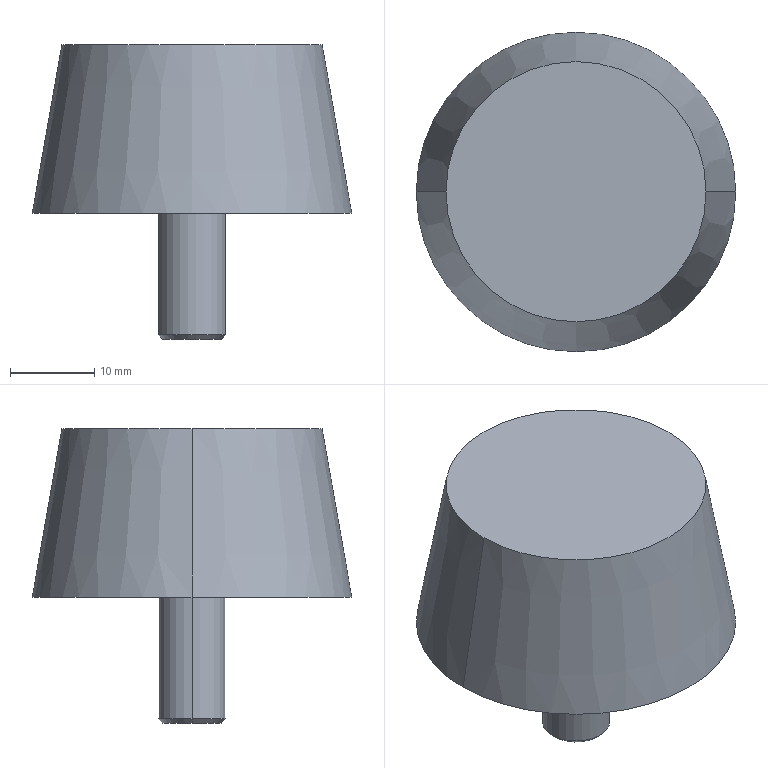Part | SolidWorks | features Chamfer 2, MoveCopyBody 2, Extrusion 1, ICE 1 | 1 solid | 9 faces | box 38 x 38 x 35 mm | volume 19484 mm3 | cone 4 | plane 3 | cylinder 2 | commonest cylinder face diameters 8 x2
STEP:
#1=CARTESIAN_POINT('',(-3.5,0.,-15.));
#2=VERTEX_POINT('',#1);
#3=CARTESIAN_POINT('',(3.5,0.,-15.));
#4=VERTEX_POINT('',#3);
#5=CARTESIAN_POINT('',(0.,0.,-15.));
#6=DIRECTION('',(0.,0.,-1.));
#7=DIRECTION('',(-1.,0.,0.));
#8=AXIS2_PLACEMENT_3D('',#5,#6,#7);
#9=CIRCLE('',#8,3.5);
#10=EDGE_CURVE('',#2,#4,#9,.T.);
#11=ORIENTED_EDGE('',*,*,#10,.F.);
#12=CARTESIAN_POINT('',(-4.,0.,-14.5));
#13=VERTEX_POINT('',#12);
#14=CARTESIAN_POINT('',(-3.5,0.,-15.));
#15=DIRECTION('',(-0.7071,0.,0.7071));
#16=VECTOR('',#15,1000.);
#17=LINE('',#14,#16);
#18=EDGE_CURVE('',#2,#13,#17,.T.);
#19=ORIENTED_EDGE('',*,*,#18,.T.);
#20=CARTESIAN_POINT('',(4.,0.,-14.5));
#21=VERTEX_POINT('',#20);
#22=CARTESIAN_POINT('',(0.,0.,-14.5));
#23=DIRECTION('',(0.,0.,1.));
#24=DIRECTION('',(-1.,0.,0.));
#25=AXIS2_PLACEMENT_3D('',#22,#23,#24);
#26=CIRCLE('',#25,4.);
#27=EDGE_CURVE('',#21,#13,#26,.T.);
#28=ORIENTED_EDGE('',*,*,#27,.F.);
#29=CARTESIAN_POINT('',(3.5,0.,-15.));
#30=DIRECTION('',(0.7071,0.,0.7071));
#31=VECTOR('',#30,1000.);
#32=LINE('',#29,#31);
#33=EDGE_CURVE('',#4,#21,#32,.T.);
#34=ORIENTED_EDGE('',*,*,#33,.F.);
#35=EDGE_LOOP('',(#11,#19,#28,#34));
#36=FACE_OUTER_BOUND('',#35,.T.);
#37=CARTESIAN_POINT('',(0.,0.,-15.));
#38=DIRECTION('',(0.,0.,1.));
#39=DIRECTION('',(1.,0.,0.));
#40=AXIS2_PLACEMENT_3D('',#37,#38,#39);
#41=CONICAL_SURFACE('',#40,3.5,0.7854);
#42=ADVANCED_FACE('',(#36),#41,.T.);
#43=ORIENTED_EDGE('',*,*,#27,.T.);
#44=CARTESIAN_POINT('',(-4.,0.,0.));
#45=VERTEX_POINT('',#44);
#46=CARTESIAN_POINT('',(-4.,0.,-15.));
#47=DIRECTION('',(0.,0.,1.));
#48=VECTOR('',#47,1000.);
#49=LINE('',#46,#48);
#50=EDGE_CURVE('',#13,#45,#49,.T.);
#51=ORIENTED_EDGE('',*,*,#50,.T.);
#52=CARTESIAN_POINT('',(4.,0.,0.));
#53=VERTEX_POINT('',#52);
#54=CARTESIAN_POINT('',(0.,0.,0.));
#55=DIRECTION('',(0.,0.,-1.));
#56=DIRECTION('',(-1.,0.,0.));
#57=AXIS2_PLACEMENT_3D('',#54,#55,#56);
#58=CIRCLE('',#57,4.);
#59=EDGE_CURVE('',#45,#53,#58,.T.);
#60=ORIENTED_EDGE('',*,*,#59,.T.);
#61=CARTESIAN_POINT('',(4.,0.,-15.));
#62=DIRECTION('',(0.,0.,1.));
#63=VECTOR('',#62,1000.);
#64=LINE('',#61,#63);
#65=EDGE_CURVE('',#21,#53,#64,.T.);
#66=ORIENTED_EDGE('',*,*,#65,.F.);
#67=EDGE_LOOP('',(#43,#51,#60,#66));
#68=FACE_OUTER_BOUND('',#67,.T.);
#69=CARTESIAN_POINT('',(0.,0.,-15.));
#70=DIRECTION('',(0.,0.,1.));
#71=DIRECTION('',(1.,0.,0.));
#72=AXIS2_PLACEMENT_3D('',#69,#70,#71);
#73=CYLINDRICAL_SURFACE('',#72,4.);
#74=ADVANCED_FACE('',(#68),#73,.T.);
#75=CARTESIAN_POINT('',(15.473,0.,20.));
#76=VERTEX_POINT('',#75);
#77=CARTESIAN_POINT('',(-15.473,0.,20.));
#78=VERTEX_POINT('',#77);
#79=CARTESIAN_POINT('',(0.,0.,20.));
#80=DIRECTION('',(0.,0.,1.));
#81=DIRECTION('',(1.,0.,0.));
#82=AXIS2_PLACEMENT_3D('',#79,#80,#81);
#83=CIRCLE('',#82,15.473);
#84=EDGE_CURVE('',#76,#78,#83,.T.);
#85=ORIENTED_EDGE('',*,*,#84,.F.);
#86=CARTESIAN_POINT('',(19.,0.,0.));
#87=VERTEX_POINT('',#86);
#88=CARTESIAN_POINT('',(15.473,0.,20.));
#89=DIRECTION('',(0.1736,0.,-0.9848));
#90=VECTOR('',#89,1000.);
#91=LINE('',#88,#90);
#92=EDGE_CURVE('',#76,#87,#91,.T.);
#93=ORIENTED_EDGE('',*,*,#92,.T.);
#94=CARTESIAN_POINT('',(-19.,0.,0.));
#95=VERTEX_POINT('',#94);
#96=CARTESIAN_POINT('',(0.,0.,0.));
#97=DIRECTION('',(0.,0.,1.));
#98=DIRECTION('',(1.,0.,0.));
#99=AXIS2_PLACEMENT_3D('',#96,#97,#98);
#100=CIRCLE('',#99,19.);
#101=EDGE_CURVE('',#87,#95,#100,.T.);
#102=ORIENTED_EDGE('',*,*,#101,.T.);
#103=CARTESIAN_POINT('',(-15.473,0.,20.));
#104=DIRECTION('',(-0.1736,0.,-0.9848));
#105=VECTOR('',#104,1000.);
#106=LINE('',#103,#105);
#107=EDGE_CURVE('',#78,#95,#106,.T.);
#108=ORIENTED_EDGE('',*,*,#107,.F.);
#109=EDGE_LOOP('',(#85,#93,#102,#108));
#110=FACE_OUTER_BOUND('',#109,.T.);
#111=CARTESIAN_POINT('',(0.,0.,20.));
#112=DIRECTION('',(0.,0.,-1.));
#113=DIRECTION('',(-1.,0.,0.));
#114=AXIS2_PLACEMENT_3D('',#111,#112,#113);
#115=CONICAL_SURFACE('',#114,15.473,0.1745);
#116=ADVANCED_FACE('',(#110),#115,.T.);
#117=CARTESIAN_POINT('',(0.,0.,20.));
#118=DIRECTION('',(0.,0.,1.));
#119=DIRECTION('',(1.,0.,0.));
#120=AXIS2_PLACEMENT_3D('',#117,#118,#119);
#121=CIRCLE('',#120,15.473);
#122=EDGE_CURVE('',#78,#76,#121,.T.);
#123=ORIENTED_EDGE('',*,*,#122,.T.);
#124=ORIENTED_EDGE('',*,*,#84,.T.);
#125=EDGE_LOOP('',(#123,#124));
#126=FACE_OUTER_BOUND('',#125,.T.);
#127=CARTESIAN_POINT('',(0.,0.,20.));
#128=DIRECTION('',(0.,0.,1.));
#129=DIRECTION('',(1.,0.,0.));
#130=AXIS2_PLACEMENT_3D('',#127,#128,#129);
#131=PLANE('',#130);
#132=ADVANCED_FACE('',(#126),#131,.T.);
#133=CARTESIAN_POINT('',(0.,0.,0.));
#134=DIRECTION('',(0.,0.,-1.));
#135=DIRECTION('',(-1.,0.,0.));
#136=AXIS2_PLACEMENT_3D('',#133,#134,#135);
#137=CIRCLE('',#136,4.);
#138=EDGE_CURVE('',#53,#45,#137,.T.);
#139=ORIENTED_EDGE('',*,*,#138,.F.);
#140=ORIENTED_EDGE('',*,*,#59,.F.);
#141=EDGE_LOOP('',(#139,#140));
#142=FACE_BOUND('',#141,.T.);
#143=CARTESIAN_POINT('',(0.,0.,0.));
#144=DIRECTION('',(0.,0.,1.));
#145=DIRECTION('',(1.,0.,0.));
#146=AXIS2_PLACEMENT_3D('',#143,#144,#145);
#147=CIRCLE('',#146,19.);
#148=EDGE_CURVE('',#95,#87,#147,.T.);
#149=ORIENTED_EDGE('',*,*,#148,.F.);
#150=ORIENTED_EDGE('',*,*,#101,.F.);
#151=EDGE_LOOP('',(#149,#150));
#152=FACE_OUTER_BOUND('',#151,.T.);
#153=CARTESIAN_POINT('',(0.,0.,0.));
#154=DIRECTION('',(0.,0.,1.));
#155=DIRECTION('',(1.,0.,0.));
#156=AXIS2_PLACEMENT_3D('',#153,#154,#155);
#157=PLANE('',#156);
#158=ADVANCED_FACE('',(#142,#152),#157,.F.);
#159=ORIENTED_EDGE('',*,*,#92,.F.);
#160=ORIENTED_EDGE('',*,*,#122,.F.);
#161=ORIENTED_EDGE('',*,*,#107,.T.);
#162=ORIENTED_EDGE('',*,*,#148,.T.);
#163=EDGE_LOOP('',(#159,#160,#161,#162));
#164=FACE_OUTER_BOUND('',#163,.T.);
#165=CARTESIAN_POINT('',(0.,0.,20.));
#166=DIRECTION('',(0.,0.,-1.));
#167=DIRECTION('',(-1.,0.,0.));
#168=AXIS2_PLACEMENT_3D('',#165,#166,#167);
#169=CONICAL_SURFACE('',#168,15.473,0.1745);
#170=ADVANCED_FACE('',(#164),#169,.T.);
#171=ORIENTED_EDGE('',*,*,#50,.F.);
#172=CARTESIAN_POINT('',(0.,0.,-14.5));
#173=DIRECTION('',(0.,0.,1.));
#174=DIRECTION('',(-1.,0.,0.));
#175=AXIS2_PLACEMENT_3D('',#172,#173,#174);
#176=CIRCLE('',#175,4.);
#177=EDGE_CURVE('',#13,#21,#176,.T.);
#178=ORIENTED_EDGE('',*,*,#177,.T.);
#179=ORIENTED_EDGE('',*,*,#65,.T.);
#180=ORIENTED_EDGE('',*,*,#138,.T.);
#181=EDGE_LOOP('',(#171,#178,#179,#180));
#182=FACE_OUTER_BOUND('',#181,.T.);
#183=CARTESIAN_POINT('',(0.,0.,-15.));
#184=DIRECTION('',(0.,0.,1.));
#185=DIRECTION('',(1.,0.,0.));
#186=AXIS2_PLACEMENT_3D('',#183,#184,#185);
#187=CYLINDRICAL_SURFACE('',#186,4.);
#188=ADVANCED_FACE('',(#182),#187,.T.);
#189=CARTESIAN_POINT('',(0.,0.,-15.));
#190=DIRECTION('',(0.,0.,-1.));
#191=DIRECTION('',(-1.,0.,0.));
#192=AXIS2_PLACEMENT_3D('',#189,#190,#191);
#193=CIRCLE('',#192,3.5);
#194=EDGE_CURVE('',#4,#2,#193,.T.);
#195=ORIENTED_EDGE('',*,*,#194,.T.);
#196=ORIENTED_EDGE('',*,*,#10,.T.);
#197=EDGE_LOOP('',(#195,#196));
#198=FACE_OUTER_BOUND('',#197,.T.);
#199=CARTESIAN_POINT('',(0.,0.,-15.));
#200=DIRECTION('',(0.,0.,-1.));
#201=DIRECTION('',(-1.,0.,0.));
#202=AXIS2_PLACEMENT_3D('',#199,#200,#201);
#203=PLANE('',#202);
#204=ADVANCED_FACE('',(#198),#203,.T.);
#205=ORIENTED_EDGE('',*,*,#18,.F.);
#206=ORIENTED_EDGE('',*,*,#194,.F.);
#207=ORIENTED_EDGE('',*,*,#33,.T.);
#208=ORIENTED_EDGE('',*,*,#177,.F.);
#209=EDGE_LOOP('',(#205,#206,#207,#208));
#210=FACE_OUTER_BOUND('',#209,.T.);
#211=CARTESIAN_POINT('',(0.,0.,-15.));
#212=DIRECTION('',(0.,0.,1.));
#213=DIRECTION('',(1.,0.,0.));
#214=AXIS2_PLACEMENT_3D('',#211,#212,#213);
#215=CONICAL_SURFACE('',#214,3.5,0.7854);
#216=ADVANCED_FACE('',(#210),#215,.T.);
#217=CLOSED_SHELL('',(#42,#74,#116,#132,#158,#170,#188,#204,#216));
#218=MANIFOLD_SOLID_BREP('',#217);
#219=CARTESIAN_POINT('',(0.,0.,0.));
#220=DIRECTION('',(0.,0.,1.));
#221=DIRECTION('',(1.,0.,0.));
#222=AXIS2_PLACEMENT_3D('',#219,#220,#221);
#223=(LENGTH_UNIT()NAMED_UNIT(*)SI_UNIT(.MILLI.,.METRE.));
#224=UNCERTAINTY_MEASURE_WITH_UNIT(LENGTH_MEASURE(0.00001),#223,'','');
#225=(NAMED_UNIT(*)PLANE_ANGLE_UNIT()SI_UNIT($,.RADIAN.));
#226=(NAMED_UNIT(*)SI_UNIT($,.STERADIAN.)SOLID_ANGLE_UNIT());
#227=(GEOMETRIC_REPRESENTATION_CONTEXT(3)GLOBAL_UNCERTAINTY_ASSIGNED_CONTEXT((#224))GLOBAL_UNIT_ASSIGNED_CONTEXT((#223,#225,#226))REPRESENTATION_CONTEXT('',''));
#228=ADVANCED_BREP_SHAPE_REPRESENTATION('',(#218,#222),#227);